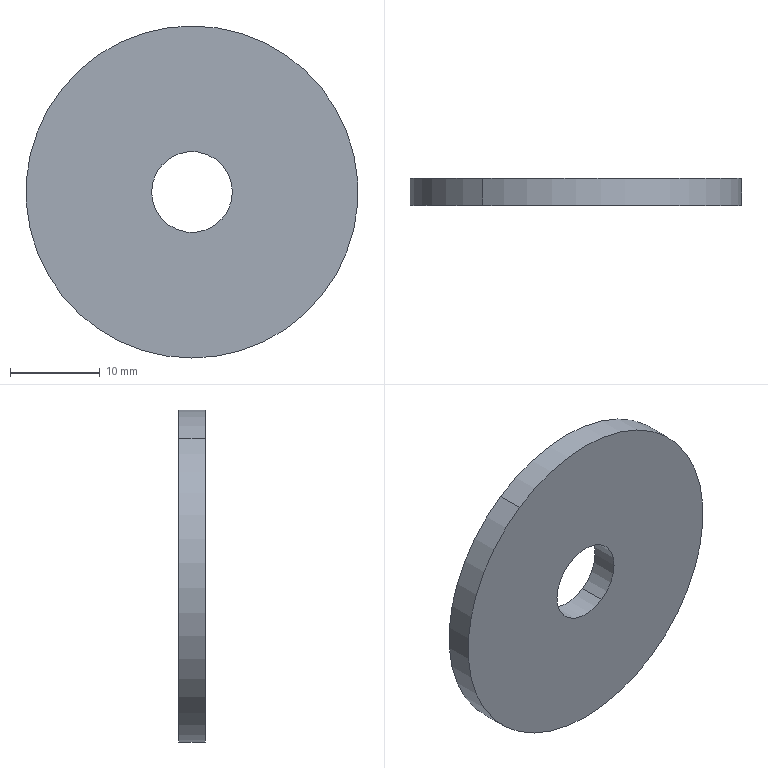Part | SolidWorks | features BaseBody 1 | 1 solid | 6 faces | box 37 x 3 x 37 mm | volume 3035 mm3 | cylinder 4 | plane 2 | commonest cylinder face diameters 9 x2 37 x2
STEP:
#1=CARTESIAN_POINT('',(-1065.487,133.946,-104.808));
#2=VERTEX_POINT('',#1);
#3=CARTESIAN_POINT('',(-1086.263,133.946,-74.192));
#4=VERTEX_POINT('',#3);
#5=CARTESIAN_POINT('',(-1075.875,133.946,-89.5));
#6=DIRECTION('',(0.,-1.,0.));
#7=DIRECTION('',(0.5615,0.,-0.8275));
#8=AXIS2_PLACEMENT_3D('',#5,#6,#7);
#9=CIRCLE('',#8,18.5);
#10=EDGE_CURVE('',#2,#4,#9,.T.);
#11=ORIENTED_EDGE('',*,*,#10,.F.);
#12=CARTESIAN_POINT('',(-1075.875,133.946,-89.5));
#13=DIRECTION('',(0.,-1.,0.));
#14=DIRECTION('',(0.5615,0.,-0.8275));
#15=AXIS2_PLACEMENT_3D('',#12,#13,#14);
#16=CIRCLE('',#15,18.5);
#17=EDGE_CURVE('',#4,#2,#16,.T.);
#18=ORIENTED_EDGE('',*,*,#17,.F.);
#19=EDGE_LOOP('',(#11,#18));
#20=FACE_OUTER_BOUND('',#19,.T.);
#21=CARTESIAN_POINT('',(-1078.402,133.946,-85.776));
#22=VERTEX_POINT('',#21);
#23=CARTESIAN_POINT('',(-1073.348,133.946,-93.224));
#24=VERTEX_POINT('',#23);
#25=CARTESIAN_POINT('',(-1075.875,133.946,-89.5));
#26=DIRECTION('',(0.,-1.,0.));
#27=DIRECTION('',(-0.5615,0.,0.8275));
#28=AXIS2_PLACEMENT_3D('',#25,#26,#27);
#29=CIRCLE('',#28,4.5);
#30=EDGE_CURVE('',#22,#24,#29,.T.);
#31=ORIENTED_EDGE('',*,*,#30,.T.);
#32=CARTESIAN_POINT('',(-1075.875,133.946,-89.5));
#33=DIRECTION('',(0.,-1.,0.));
#34=DIRECTION('',(-0.5615,0.,0.8275));
#35=AXIS2_PLACEMENT_3D('',#32,#33,#34);
#36=CIRCLE('',#35,4.5);
#37=EDGE_CURVE('',#24,#22,#36,.T.);
#38=ORIENTED_EDGE('',*,*,#37,.T.);
#39=EDGE_LOOP('',(#31,#38));
#40=FACE_BOUND('',#39,.T.);
#41=CARTESIAN_POINT('',(-1075.875,133.946,-89.5));
#42=DIRECTION('',(0.,-1.,0.));
#43=DIRECTION('',(-0.8275,0.,-0.5615));
#44=AXIS2_PLACEMENT_3D('',#41,#42,#43);
#45=PLANE('',#44);
#46=ADVANCED_FACE('',(#20,#40),#45,.F.);
#47=CARTESIAN_POINT('',(-1073.348,130.946,-93.224));
#48=VERTEX_POINT('',#47);
#49=CARTESIAN_POINT('',(-1073.348,133.946,-93.224));
#50=DIRECTION('',(0.,-1.,0.));
#51=VECTOR('',#50,1000.);
#52=LINE('',#49,#51);
#53=EDGE_CURVE('',#24,#48,#52,.T.);
#54=ORIENTED_EDGE('',*,*,#53,.F.);
#55=ORIENTED_EDGE('',*,*,#30,.F.);
#56=CARTESIAN_POINT('',(-1078.402,130.946,-85.776));
#57=VERTEX_POINT('',#56);
#58=CARTESIAN_POINT('',(-1078.402,133.946,-85.776));
#59=DIRECTION('',(0.,-1.,0.));
#60=VECTOR('',#59,1000.);
#61=LINE('',#58,#60);
#62=EDGE_CURVE('',#22,#57,#61,.T.);
#63=ORIENTED_EDGE('',*,*,#62,.T.);
#64=CARTESIAN_POINT('',(-1075.875,130.946,-89.5));
#65=DIRECTION('',(0.,1.,0.));
#66=DIRECTION('',(-0.5615,0.,0.8275));
#67=AXIS2_PLACEMENT_3D('',#64,#65,#66);
#68=CIRCLE('',#67,4.5);
#69=EDGE_CURVE('',#48,#57,#68,.T.);
#70=ORIENTED_EDGE('',*,*,#69,.F.);
#71=EDGE_LOOP('',(#54,#55,#63,#70));
#72=FACE_OUTER_BOUND('',#71,.T.);
#73=CARTESIAN_POINT('',(-1075.875,133.946,-89.5));
#74=DIRECTION('',(0.,-1.,0.));
#75=DIRECTION('',(-0.5615,0.,0.8275));
#76=AXIS2_PLACEMENT_3D('',#73,#74,#75);
#77=CYLINDRICAL_SURFACE('',#76,4.5);
#78=ADVANCED_FACE('',(#72),#77,.F.);
#79=CARTESIAN_POINT('',(-1086.263,130.946,-74.192));
#80=VERTEX_POINT('',#79);
#81=CARTESIAN_POINT('',(-1086.263,130.946,-74.192));
#82=DIRECTION('',(0.,1.,0.));
#83=VECTOR('',#82,1000.);
#84=LINE('',#81,#83);
#85=EDGE_CURVE('',#80,#4,#84,.T.);
#86=ORIENTED_EDGE('',*,*,#85,.F.);
#87=CARTESIAN_POINT('',(-1065.487,130.946,-104.808));
#88=VERTEX_POINT('',#87);
#89=CARTESIAN_POINT('',(-1075.875,130.946,-89.5));
#90=DIRECTION('',(0.,-1.,0.));
#91=DIRECTION('',(0.5615,0.,-0.8275));
#92=AXIS2_PLACEMENT_3D('',#89,#90,#91);
#93=CIRCLE('',#92,18.5);
#94=EDGE_CURVE('',#88,#80,#93,.T.);
#95=ORIENTED_EDGE('',*,*,#94,.F.);
#96=CARTESIAN_POINT('',(-1065.487,130.946,-104.808));
#97=DIRECTION('',(0.,1.,0.));
#98=VECTOR('',#97,1000.);
#99=LINE('',#96,#98);
#100=EDGE_CURVE('',#88,#2,#99,.T.);
#101=ORIENTED_EDGE('',*,*,#100,.T.);
#102=ORIENTED_EDGE('',*,*,#10,.T.);
#103=EDGE_LOOP('',(#86,#95,#101,#102));
#104=FACE_OUTER_BOUND('',#103,.T.);
#105=CARTESIAN_POINT('',(-1075.875,130.946,-89.5));
#106=DIRECTION('',(0.,1.,0.));
#107=DIRECTION('',(0.5615,0.,-0.8275));
#108=AXIS2_PLACEMENT_3D('',#105,#106,#107);
#109=CYLINDRICAL_SURFACE('',#108,18.5);
#110=ADVANCED_FACE('',(#104),#109,.T.);
#111=ORIENTED_EDGE('',*,*,#94,.T.);
#112=CARTESIAN_POINT('',(-1075.875,130.946,-89.5));
#113=DIRECTION('',(0.,-1.,0.));
#114=DIRECTION('',(0.5615,0.,-0.8275));
#115=AXIS2_PLACEMENT_3D('',#112,#113,#114);
#116=CIRCLE('',#115,18.5);
#117=EDGE_CURVE('',#80,#88,#116,.T.);
#118=ORIENTED_EDGE('',*,*,#117,.T.);
#119=EDGE_LOOP('',(#111,#118));
#120=FACE_OUTER_BOUND('',#119,.T.);
#121=CARTESIAN_POINT('',(-1075.875,130.946,-89.5));
#122=DIRECTION('',(0.,1.,0.));
#123=DIRECTION('',(-0.5615,0.,0.8275));
#124=AXIS2_PLACEMENT_3D('',#121,#122,#123);
#125=CIRCLE('',#124,4.5);
#126=EDGE_CURVE('',#57,#48,#125,.T.);
#127=ORIENTED_EDGE('',*,*,#126,.T.);
#128=ORIENTED_EDGE('',*,*,#69,.T.);
#129=EDGE_LOOP('',(#127,#128));
#130=FACE_BOUND('',#129,.T.);
#131=CARTESIAN_POINT('',(-1075.875,130.946,-89.5));
#132=DIRECTION('',(0.,-1.,0.));
#133=DIRECTION('',(-0.8275,0.,-0.5615));
#134=AXIS2_PLACEMENT_3D('',#131,#132,#133);
#135=PLANE('',#134);
#136=ADVANCED_FACE('',(#120,#130),#135,.T.);
#137=ORIENTED_EDGE('',*,*,#37,.F.);
#138=ORIENTED_EDGE('',*,*,#53,.T.);
#139=ORIENTED_EDGE('',*,*,#126,.F.);
#140=ORIENTED_EDGE('',*,*,#62,.F.);
#141=EDGE_LOOP('',(#137,#138,#139,#140));
#142=FACE_OUTER_BOUND('',#141,.T.);
#143=CARTESIAN_POINT('',(-1075.875,133.946,-89.5));
#144=DIRECTION('',(0.,-1.,0.));
#145=DIRECTION('',(-0.5615,0.,0.8275));
#146=AXIS2_PLACEMENT_3D('',#143,#144,#145);
#147=CYLINDRICAL_SURFACE('',#146,4.5);
#148=ADVANCED_FACE('',(#142),#147,.F.);
#149=ORIENTED_EDGE('',*,*,#117,.F.);
#150=ORIENTED_EDGE('',*,*,#85,.T.);
#151=ORIENTED_EDGE('',*,*,#17,.T.);
#152=ORIENTED_EDGE('',*,*,#100,.F.);
#153=EDGE_LOOP('',(#149,#150,#151,#152));
#154=FACE_OUTER_BOUND('',#153,.T.);
#155=CARTESIAN_POINT('',(-1075.875,130.946,-89.5));
#156=DIRECTION('',(0.,1.,0.));
#157=DIRECTION('',(0.5615,0.,-0.8275));
#158=AXIS2_PLACEMENT_3D('',#155,#156,#157);
#159=CYLINDRICAL_SURFACE('',#158,18.5);
#160=ADVANCED_FACE('',(#154),#159,.T.);
#161=CLOSED_SHELL('',(#46,#78,#110,#136,#148,#160));
#162=MANIFOLD_SOLID_BREP('',#161);
#163=CARTESIAN_POINT('',(0.,0.,0.));
#164=DIRECTION('',(0.,0.,1.));
#165=DIRECTION('',(1.,0.,0.));
#166=AXIS2_PLACEMENT_3D('',#163,#164,#165);
#167=(LENGTH_UNIT()NAMED_UNIT(*)SI_UNIT(.MILLI.,.METRE.));
#168=UNCERTAINTY_MEASURE_WITH_UNIT(LENGTH_MEASURE(0.00001),#167,'','');
#169=(NAMED_UNIT(*)PLANE_ANGLE_UNIT()SI_UNIT($,.RADIAN.));
#170=(NAMED_UNIT(*)SI_UNIT($,.STERADIAN.)SOLID_ANGLE_UNIT());
#171=(GEOMETRIC_REPRESENTATION_CONTEXT(3)GLOBAL_UNCERTAINTY_ASSIGNED_CONTEXT((#168))GLOBAL_UNIT_ASSIGNED_CONTEXT((#167,#169,#170))REPRESENTATION_CONTEXT('',''));
#172=ADVANCED_BREP_SHAPE_REPRESENTATION('',(#162,#166),#171);